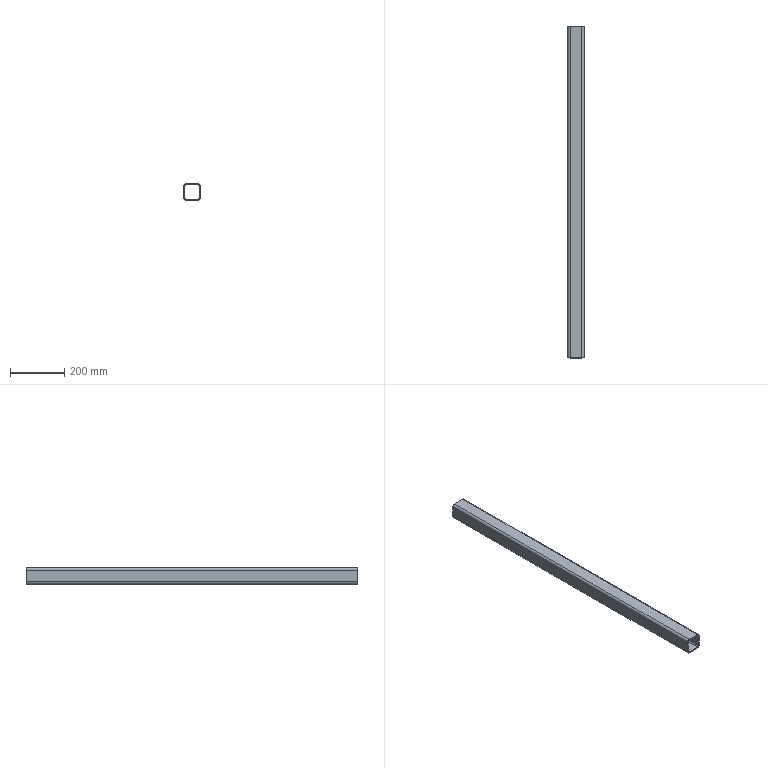Part | SolidWorks | features BaseBody 1 | 1 solid | 18 faces | box 60 x 1220 x 60 mm | volume 1042852 mm3 | plane 10 | cylinder 8 | commonest cylinder face diameters 8 x4 16 x4
STEP:
#1=CARTESIAN_POINT('',(-644.,2432.,552.));
#2=VERTEX_POINT('',#1);
#3=CARTESIAN_POINT('',(-644.,2432.,508.));
#4=VERTEX_POINT('',#3);
#5=CARTESIAN_POINT('',(-644.,2432.,508.));
#6=DIRECTION('',(0.,0.,-1.));
#7=VECTOR('',#6,1000.);
#8=LINE('',#5,#7);
#9=EDGE_CURVE('',#2,#4,#8,.T.);
#10=ORIENTED_EDGE('',*,*,#9,.T.);
#11=CARTESIAN_POINT('',(-644.,1212.,508.));
#12=VERTEX_POINT('',#11);
#13=CARTESIAN_POINT('',(-644.,2462.,508.));
#14=DIRECTION('',(0.,-1.,0.));
#15=VECTOR('',#14,1000.);
#16=LINE('',#13,#15);
#17=EDGE_CURVE('',#4,#12,#16,.T.);
#18=ORIENTED_EDGE('',*,*,#17,.T.);
#19=CARTESIAN_POINT('',(-644.,1212.,552.));
#20=VERTEX_POINT('',#19);
#21=CARTESIAN_POINT('',(-644.,1212.,508.));
#22=DIRECTION('',(0.,0.,1.));
#23=VECTOR('',#22,1000.);
#24=LINE('',#21,#23);
#25=EDGE_CURVE('',#12,#20,#24,.T.);
#26=ORIENTED_EDGE('',*,*,#25,.T.);
#27=CARTESIAN_POINT('',(-644.,2462.,552.));
#28=DIRECTION('',(0.,1.,0.));
#29=VECTOR('',#28,1000.);
#30=LINE('',#27,#29);
#31=EDGE_CURVE('',#20,#2,#30,.T.);
#32=ORIENTED_EDGE('',*,*,#31,.T.);
#33=EDGE_LOOP('',(#10,#18,#26,#32));
#34=FACE_OUTER_BOUND('',#33,.T.);
#35=CARTESIAN_POINT('',(-644.,2462.,508.));
#36=DIRECTION('',(-1.,0.,0.));
#37=DIRECTION('',(0.,0.,1.));
#38=AXIS2_PLACEMENT_3D('',#35,#36,#37);
#39=PLANE('',#38);
#40=ADVANCED_FACE('',(#34),#39,.T.);
#41=ORIENTED_EDGE('',*,*,#17,.F.);
#42=CARTESIAN_POINT('',(-648.,2432.,504.));
#43=VERTEX_POINT('',#42);
#44=CARTESIAN_POINT('',(-648.,2432.,508.));
#45=DIRECTION('',(0.,-1.,0.));
#46=DIRECTION('',(0.,0.,-1.));
#47=AXIS2_PLACEMENT_3D('',#44,#45,#46);
#48=CIRCLE('',#47,4.);
#49=EDGE_CURVE('',#43,#4,#48,.T.);
#50=ORIENTED_EDGE('',*,*,#49,.F.);
#51=CARTESIAN_POINT('',(-648.,1212.,504.));
#52=VERTEX_POINT('',#51);
#53=CARTESIAN_POINT('',(-648.,2462.,504.));
#54=DIRECTION('',(0.,1.,0.));
#55=VECTOR('',#54,1000.);
#56=LINE('',#53,#55);
#57=EDGE_CURVE('',#52,#43,#56,.T.);
#58=ORIENTED_EDGE('',*,*,#57,.F.);
#59=CARTESIAN_POINT('',(-648.,1212.,508.));
#60=DIRECTION('',(0.,1.,0.));
#61=DIRECTION('',(0.,0.,-1.));
#62=AXIS2_PLACEMENT_3D('',#59,#60,#61);
#63=CIRCLE('',#62,4.);
#64=EDGE_CURVE('',#12,#52,#63,.T.);
#65=ORIENTED_EDGE('',*,*,#64,.F.);
#66=EDGE_LOOP('',(#41,#50,#58,#65));
#67=FACE_OUTER_BOUND('',#66,.T.);
#68=CARTESIAN_POINT('',(-648.,2462.,508.));
#69=DIRECTION('',(0.,-1.,0.));
#70=DIRECTION('',(0.,0.,-1.));
#71=AXIS2_PLACEMENT_3D('',#68,#69,#70);
#72=CYLINDRICAL_SURFACE('',#71,4.);
#73=ADVANCED_FACE('',(#67),#72,.F.);
#74=CARTESIAN_POINT('',(-648.,2432.,556.));
#75=VERTEX_POINT('',#74);
#76=CARTESIAN_POINT('',(-648.,2432.,552.));
#77=DIRECTION('',(0.,-1.,0.));
#78=DIRECTION('',(0.,0.,-1.));
#79=AXIS2_PLACEMENT_3D('',#76,#77,#78);
#80=CIRCLE('',#79,4.);
#81=EDGE_CURVE('',#2,#75,#80,.T.);
#82=ORIENTED_EDGE('',*,*,#81,.T.);
#83=CARTESIAN_POINT('',(-692.,2432.,556.));
#84=VERTEX_POINT('',#83);
#85=CARTESIAN_POINT('',(-648.,2432.,556.));
#86=DIRECTION('',(-1.,0.,0.));
#87=VECTOR('',#86,1000.);
#88=LINE('',#85,#87);
#89=EDGE_CURVE('',#75,#84,#88,.T.);
#90=ORIENTED_EDGE('',*,*,#89,.T.);
#91=CARTESIAN_POINT('',(-696.,2432.,552.));
#92=VERTEX_POINT('',#91);
#93=CARTESIAN_POINT('',(-692.,2432.,552.));
#94=DIRECTION('',(0.,-1.,0.));
#95=DIRECTION('',(0.,0.,-1.));
#96=AXIS2_PLACEMENT_3D('',#93,#94,#95);
#97=CIRCLE('',#96,4.);
#98=EDGE_CURVE('',#84,#92,#97,.T.);
#99=ORIENTED_EDGE('',*,*,#98,.T.);
#100=CARTESIAN_POINT('',(-696.,2432.,508.));
#101=VERTEX_POINT('',#100);
#102=CARTESIAN_POINT('',(-696.,2432.,-1270.));
#103=DIRECTION('',(0.,0.,-1.));
#104=VECTOR('',#103,1000.);
#105=LINE('',#102,#104);
#106=EDGE_CURVE('',#92,#101,#105,.T.);
#107=ORIENTED_EDGE('',*,*,#106,.T.);
#108=CARTESIAN_POINT('',(-692.,2432.,504.));
#109=VERTEX_POINT('',#108);
#110=CARTESIAN_POINT('',(-692.,2432.,508.));
#111=DIRECTION('',(0.,-1.,0.));
#112=DIRECTION('',(0.,0.,-1.));
#113=AXIS2_PLACEMENT_3D('',#110,#111,#112);
#114=CIRCLE('',#113,4.);
#115=EDGE_CURVE('',#101,#109,#114,.T.);
#116=ORIENTED_EDGE('',*,*,#115,.T.);
#117=CARTESIAN_POINT('',(-648.,2432.,504.));
#118=DIRECTION('',(1.,0.,0.));
#119=VECTOR('',#118,1000.);
#120=LINE('',#117,#119);
#121=EDGE_CURVE('',#109,#43,#120,.T.);
#122=ORIENTED_EDGE('',*,*,#121,.T.);
#123=ORIENTED_EDGE('',*,*,#49,.T.);
#124=ORIENTED_EDGE('',*,*,#9,.F.);
#125=EDGE_LOOP('',(#82,#90,#99,#107,#116,#122,#123,#124));
#126=FACE_BOUND('',#125,.T.);
#127=CARTESIAN_POINT('',(-700.,2432.,508.));
#128=VERTEX_POINT('',#127);
#129=CARTESIAN_POINT('',(-700.,2432.,552.));
#130=VERTEX_POINT('',#129);
#131=CARTESIAN_POINT('',(-700.,2432.,-1270.));
#132=DIRECTION('',(0.,0.,1.));
#133=VECTOR('',#132,1000.);
#134=LINE('',#131,#133);
#135=EDGE_CURVE('',#128,#130,#134,.T.);
#136=ORIENTED_EDGE('',*,*,#135,.T.);
#137=CARTESIAN_POINT('',(-692.,2432.,560.));
#138=VERTEX_POINT('',#137);
#139=CARTESIAN_POINT('',(-692.,2432.,552.));
#140=DIRECTION('',(0.,1.,0.));
#141=DIRECTION('',(0.,0.,-1.));
#142=AXIS2_PLACEMENT_3D('',#139,#140,#141);
#143=CIRCLE('',#142,8.);
#144=EDGE_CURVE('',#130,#138,#143,.T.);
#145=ORIENTED_EDGE('',*,*,#144,.T.);
#146=CARTESIAN_POINT('',(-648.,2432.,560.));
#147=VERTEX_POINT('',#146);
#148=CARTESIAN_POINT('',(-648.,2432.,560.));
#149=DIRECTION('',(1.,0.,0.));
#150=VECTOR('',#149,1000.);
#151=LINE('',#148,#150);
#152=EDGE_CURVE('',#138,#147,#151,.T.);
#153=ORIENTED_EDGE('',*,*,#152,.T.);
#154=CARTESIAN_POINT('',(-640.,2432.,552.));
#155=VERTEX_POINT('',#154);
#156=CARTESIAN_POINT('',(-648.,2432.,552.));
#157=DIRECTION('',(0.,1.,0.));
#158=DIRECTION('',(0.,0.,-1.));
#159=AXIS2_PLACEMENT_3D('',#156,#157,#158);
#160=CIRCLE('',#159,8.);
#161=EDGE_CURVE('',#147,#155,#160,.T.);
#162=ORIENTED_EDGE('',*,*,#161,.T.);
#163=CARTESIAN_POINT('',(-640.,2432.,508.));
#164=VERTEX_POINT('',#163);
#165=CARTESIAN_POINT('',(-640.,2432.,-1270.));
#166=DIRECTION('',(0.,0.,-1.));
#167=VECTOR('',#166,1000.);
#168=LINE('',#165,#167);
#169=EDGE_CURVE('',#155,#164,#168,.T.);
#170=ORIENTED_EDGE('',*,*,#169,.T.);
#171=CARTESIAN_POINT('',(-648.,2432.,500.));
#172=VERTEX_POINT('',#171);
#173=CARTESIAN_POINT('',(-648.,2432.,508.));
#174=DIRECTION('',(0.,1.,0.));
#175=DIRECTION('',(0.,0.,-1.));
#176=AXIS2_PLACEMENT_3D('',#173,#174,#175);
#177=CIRCLE('',#176,8.);
#178=EDGE_CURVE('',#164,#172,#177,.T.);
#179=ORIENTED_EDGE('',*,*,#178,.T.);
#180=CARTESIAN_POINT('',(-692.,2432.,500.));
#181=VERTEX_POINT('',#180);
#182=CARTESIAN_POINT('',(-648.,2432.,500.));
#183=DIRECTION('',(-1.,0.,0.));
#184=VECTOR('',#183,1000.);
#185=LINE('',#182,#184);
#186=EDGE_CURVE('',#172,#181,#185,.T.);
#187=ORIENTED_EDGE('',*,*,#186,.T.);
#188=CARTESIAN_POINT('',(-692.,2432.,508.));
#189=DIRECTION('',(0.,1.,0.));
#190=DIRECTION('',(0.,0.,-1.));
#191=AXIS2_PLACEMENT_3D('',#188,#189,#190);
#192=CIRCLE('',#191,8.);
#193=EDGE_CURVE('',#181,#128,#192,.T.);
#194=ORIENTED_EDGE('',*,*,#193,.T.);
#195=EDGE_LOOP('',(#136,#145,#153,#162,#170,#179,#187,#194));
#196=FACE_OUTER_BOUND('',#195,.T.);
#197=CARTESIAN_POINT('',(-648.,2432.,-1270.));
#198=DIRECTION('',(0.,1.,0.));
#199=DIRECTION('',(0.,0.,1.));
#200=AXIS2_PLACEMENT_3D('',#197,#198,#199);
#201=PLANE('',#200);
#202=ADVANCED_FACE('',(#126,#196),#201,.T.);
#203=CARTESIAN_POINT('',(-648.,1212.,556.));
#204=VERTEX_POINT('',#203);
#205=CARTESIAN_POINT('',(-648.,2462.,556.));
#206=DIRECTION('',(0.,-1.,0.));
#207=VECTOR('',#206,1000.);
#208=LINE('',#205,#207);
#209=EDGE_CURVE('',#75,#204,#208,.T.);
#210=ORIENTED_EDGE('',*,*,#209,.F.);
#211=ORIENTED_EDGE('',*,*,#81,.F.);
#212=ORIENTED_EDGE('',*,*,#31,.F.);
#213=CARTESIAN_POINT('',(-648.,1212.,552.));
#214=DIRECTION('',(0.,1.,0.));
#215=DIRECTION('',(0.,0.,-1.));
#216=AXIS2_PLACEMENT_3D('',#213,#214,#215);
#217=CIRCLE('',#216,4.);
#218=EDGE_CURVE('',#204,#20,#217,.T.);
#219=ORIENTED_EDGE('',*,*,#218,.F.);
#220=EDGE_LOOP('',(#210,#211,#212,#219));
#221=FACE_OUTER_BOUND('',#220,.T.);
#222=CARTESIAN_POINT('',(-648.,2462.,552.));
#223=DIRECTION('',(0.,-1.,0.));
#224=DIRECTION('',(0.,0.,-1.));
#225=AXIS2_PLACEMENT_3D('',#222,#223,#224);
#226=CYLINDRICAL_SURFACE('',#225,4.);
#227=ADVANCED_FACE('',(#221),#226,.F.);
#228=CARTESIAN_POINT('',(-692.,1212.,556.));
#229=VERTEX_POINT('',#228);
#230=CARTESIAN_POINT('',(-640.,1212.,556.));
#231=DIRECTION('',(1.,0.,0.));
#232=VECTOR('',#231,1000.);
#233=LINE('',#230,#232);
#234=EDGE_CURVE('',#229,#204,#233,.T.);
#235=ORIENTED_EDGE('',*,*,#234,.T.);
#236=ORIENTED_EDGE('',*,*,#218,.T.);
#237=ORIENTED_EDGE('',*,*,#25,.F.);
#238=ORIENTED_EDGE('',*,*,#64,.T.);
#239=CARTESIAN_POINT('',(-692.,1212.,504.));
#240=VERTEX_POINT('',#239);
#241=CARTESIAN_POINT('',(-640.,1212.,504.));
#242=DIRECTION('',(-1.,0.,0.));
#243=VECTOR('',#242,1000.);
#244=LINE('',#241,#243);
#245=EDGE_CURVE('',#52,#240,#244,.T.);
#246=ORIENTED_EDGE('',*,*,#245,.T.);
#247=CARTESIAN_POINT('',(-696.,1212.,508.));
#248=VERTEX_POINT('',#247);
#249=CARTESIAN_POINT('',(-692.,1212.,508.));
#250=DIRECTION('',(0.,1.,0.));
#251=DIRECTION('',(0.,0.,-1.));
#252=AXIS2_PLACEMENT_3D('',#249,#250,#251);
#253=CIRCLE('',#252,4.);
#254=EDGE_CURVE('',#240,#248,#253,.T.);
#255=ORIENTED_EDGE('',*,*,#254,.T.);
#256=CARTESIAN_POINT('',(-696.,1212.,552.));
#257=VERTEX_POINT('',#256);
#258=CARTESIAN_POINT('',(-696.,1212.,530.));
#259=DIRECTION('',(0.,0.,1.));
#260=VECTOR('',#259,1000.);
#261=LINE('',#258,#260);
#262=EDGE_CURVE('',#248,#257,#261,.T.);
#263=ORIENTED_EDGE('',*,*,#262,.T.);
#264=CARTESIAN_POINT('',(-692.,1212.,552.));
#265=DIRECTION('',(0.,1.,0.));
#266=DIRECTION('',(0.,0.,-1.));
#267=AXIS2_PLACEMENT_3D('',#264,#265,#266);
#268=CIRCLE('',#267,4.);
#269=EDGE_CURVE('',#257,#229,#268,.T.);
#270=ORIENTED_EDGE('',*,*,#269,.T.);
#271=EDGE_LOOP('',(#235,#236,#237,#238,#246,#255,#263,#270));
#272=FACE_BOUND('',#271,.T.);
#273=CARTESIAN_POINT('',(-640.,1212.,552.));
#274=VERTEX_POINT('',#273);
#275=CARTESIAN_POINT('',(-648.,1212.,560.));
#276=VERTEX_POINT('',#275);
#277=CARTESIAN_POINT('',(-648.,1212.,552.));
#278=DIRECTION('',(0.,-1.,0.));
#279=DIRECTION('',(0.,0.,-1.));
#280=AXIS2_PLACEMENT_3D('',#277,#278,#279);
#281=CIRCLE('',#280,8.);
#282=EDGE_CURVE('',#274,#276,#281,.T.);
#283=ORIENTED_EDGE('',*,*,#282,.T.);
#284=CARTESIAN_POINT('',(-692.,1212.,560.));
#285=VERTEX_POINT('',#284);
#286=CARTESIAN_POINT('',(-640.,1212.,560.));
#287=DIRECTION('',(-1.,0.,0.));
#288=VECTOR('',#287,1000.);
#289=LINE('',#286,#288);
#290=EDGE_CURVE('',#276,#285,#289,.T.);
#291=ORIENTED_EDGE('',*,*,#290,.T.);
#292=CARTESIAN_POINT('',(-700.,1212.,552.));
#293=VERTEX_POINT('',#292);
#294=CARTESIAN_POINT('',(-692.,1212.,552.));
#295=DIRECTION('',(0.,-1.,0.));
#296=DIRECTION('',(0.,0.,-1.));
#297=AXIS2_PLACEMENT_3D('',#294,#295,#296);
#298=CIRCLE('',#297,8.);
#299=EDGE_CURVE('',#285,#293,#298,.T.);
#300=ORIENTED_EDGE('',*,*,#299,.T.);
#301=CARTESIAN_POINT('',(-700.,1212.,508.));
#302=VERTEX_POINT('',#301);
#303=CARTESIAN_POINT('',(-700.,1212.,530.));
#304=DIRECTION('',(0.,0.,-1.));
#305=VECTOR('',#304,1000.);
#306=LINE('',#303,#305);
#307=EDGE_CURVE('',#293,#302,#306,.T.);
#308=ORIENTED_EDGE('',*,*,#307,.T.);
#309=CARTESIAN_POINT('',(-692.,1212.,500.));
#310=VERTEX_POINT('',#309);
#311=CARTESIAN_POINT('',(-692.,1212.,508.));
#312=DIRECTION('',(0.,-1.,0.));
#313=DIRECTION('',(0.,0.,-1.));
#314=AXIS2_PLACEMENT_3D('',#311,#312,#313);
#315=CIRCLE('',#314,8.);
#316=EDGE_CURVE('',#302,#310,#315,.T.);
#317=ORIENTED_EDGE('',*,*,#316,.T.);
#318=CARTESIAN_POINT('',(-648.,1212.,500.));
#319=VERTEX_POINT('',#318);
#320=CARTESIAN_POINT('',(-640.,1212.,500.));
#321=DIRECTION('',(1.,0.,0.));
#322=VECTOR('',#321,1000.);
#323=LINE('',#320,#322);
#324=EDGE_CURVE('',#310,#319,#323,.T.);
#325=ORIENTED_EDGE('',*,*,#324,.T.);
#326=CARTESIAN_POINT('',(-640.,1212.,508.));
#327=VERTEX_POINT('',#326);
#328=CARTESIAN_POINT('',(-648.,1212.,508.));
#329=DIRECTION('',(0.,-1.,0.));
#330=DIRECTION('',(0.,0.,-1.));
#331=AXIS2_PLACEMENT_3D('',#328,#329,#330);
#332=CIRCLE('',#331,8.);
#333=EDGE_CURVE('',#319,#327,#332,.T.);
#334=ORIENTED_EDGE('',*,*,#333,.T.);
#335=CARTESIAN_POINT('',(-640.,1212.,530.));
#336=DIRECTION('',(0.,0.,1.));
#337=VECTOR('',#336,1000.);
#338=LINE('',#335,#337);
#339=EDGE_CURVE('',#327,#274,#338,.T.);
#340=ORIENTED_EDGE('',*,*,#339,.T.);
#341=EDGE_LOOP('',(#283,#291,#300,#308,#317,#325,#334,#340));
#342=FACE_OUTER_BOUND('',#341,.T.);
#343=CARTESIAN_POINT('',(-640.,1212.,530.));
#344=DIRECTION('',(0.,-1.,0.));
#345=DIRECTION('',(0.,0.,-1.));
#346=AXIS2_PLACEMENT_3D('',#343,#344,#345);
#347=PLANE('',#346);
#348=ADVANCED_FACE('',(#272,#342),#347,.T.);
#349=ORIENTED_EDGE('',*,*,#121,.F.);
#350=CARTESIAN_POINT('',(-692.,2462.,504.));
#351=DIRECTION('',(0.,-1.,0.));
#352=VECTOR('',#351,1000.);
#353=LINE('',#350,#352);
#354=EDGE_CURVE('',#109,#240,#353,.T.);
#355=ORIENTED_EDGE('',*,*,#354,.T.);
#356=ORIENTED_EDGE('',*,*,#245,.F.);
#357=ORIENTED_EDGE('',*,*,#57,.T.);
#358=EDGE_LOOP('',(#349,#355,#356,#357));
#359=FACE_OUTER_BOUND('',#358,.T.);
#360=CARTESIAN_POINT('',(-648.,2462.,504.));
#361=DIRECTION('',(0.,0.,1.));
#362=DIRECTION('',(1.,0.,0.));
#363=AXIS2_PLACEMENT_3D('',#360,#361,#362);
#364=PLANE('',#363);
#365=ADVANCED_FACE('',(#359),#364,.T.);
#366=ORIENTED_EDGE('',*,*,#89,.F.);
#367=ORIENTED_EDGE('',*,*,#209,.T.);
#368=ORIENTED_EDGE('',*,*,#234,.F.);
#369=CARTESIAN_POINT('',(-692.,2462.,556.));
#370=DIRECTION('',(0.,1.,0.));
#371=VECTOR('',#370,1000.);
#372=LINE('',#369,#371);
#373=EDGE_CURVE('',#229,#84,#372,.T.);
#374=ORIENTED_EDGE('',*,*,#373,.T.);
#375=EDGE_LOOP('',(#366,#367,#368,#374));
#376=FACE_OUTER_BOUND('',#375,.T.);
#377=CARTESIAN_POINT('',(-692.,2462.,556.));
#378=DIRECTION('',(0.,0.,-1.));
#379=DIRECTION('',(-1.,0.,0.));
#380=AXIS2_PLACEMENT_3D('',#377,#378,#379);
#381=PLANE('',#380);
#382=ADVANCED_FACE('',(#376),#381,.T.);
#383=ORIENTED_EDGE('',*,*,#354,.F.);
#384=ORIENTED_EDGE('',*,*,#115,.F.);
#385=CARTESIAN_POINT('',(-696.,2462.,508.));
#386=DIRECTION('',(0.,1.,0.));
#387=VECTOR('',#386,1000.);
#388=LINE('',#385,#387);
#389=EDGE_CURVE('',#248,#101,#388,.T.);
#390=ORIENTED_EDGE('',*,*,#389,.F.);
#391=ORIENTED_EDGE('',*,*,#254,.F.);
#392=EDGE_LOOP('',(#383,#384,#390,#391));
#393=FACE_OUTER_BOUND('',#392,.T.);
#394=CARTESIAN_POINT('',(-692.,2462.,508.));
#395=DIRECTION('',(0.,-1.,0.));
#396=DIRECTION('',(0.,0.,-1.));
#397=AXIS2_PLACEMENT_3D('',#394,#395,#396);
#398=CYLINDRICAL_SURFACE('',#397,4.);
#399=ADVANCED_FACE('',(#393),#398,.F.);
#400=ORIENTED_EDGE('',*,*,#106,.F.);
#401=CARTESIAN_POINT('',(-696.,2462.,552.));
#402=DIRECTION('',(0.,-1.,0.));
#403=VECTOR('',#402,1000.);
#404=LINE('',#401,#403);
#405=EDGE_CURVE('',#92,#257,#404,.T.);
#406=ORIENTED_EDGE('',*,*,#405,.T.);
#407=ORIENTED_EDGE('',*,*,#262,.F.);
#408=ORIENTED_EDGE('',*,*,#389,.T.);
#409=EDGE_LOOP('',(#400,#406,#407,#408));
#410=FACE_OUTER_BOUND('',#409,.T.);
#411=CARTESIAN_POINT('',(-696.,2462.,552.));
#412=DIRECTION('',(1.,0.,0.));
#413=DIRECTION('',(0.,0.,-1.));
#414=AXIS2_PLACEMENT_3D('',#411,#412,#413);
#415=PLANE('',#414);
#416=ADVANCED_FACE('',(#410),#415,.T.);
#417=ORIENTED_EDGE('',*,*,#405,.F.);
#418=ORIENTED_EDGE('',*,*,#98,.F.);
#419=ORIENTED_EDGE('',*,*,#373,.F.);
#420=ORIENTED_EDGE('',*,*,#269,.F.);
#421=EDGE_LOOP('',(#417,#418,#419,#420));
#422=FACE_OUTER_BOUND('',#421,.T.);
#423=CARTESIAN_POINT('',(-692.,2462.,552.));
#424=DIRECTION('',(0.,-1.,0.));
#425=DIRECTION('',(0.,0.,-1.));
#426=AXIS2_PLACEMENT_3D('',#423,#424,#425);
#427=CYLINDRICAL_SURFACE('',#426,4.);
#428=ADVANCED_FACE('',(#422),#427,.F.);
#429=CARTESIAN_POINT('',(-700.,2462.,552.));
#430=DIRECTION('',(0.,-1.,0.));
#431=VECTOR('',#430,1000.);
#432=LINE('',#429,#431);
#433=EDGE_CURVE('',#130,#293,#432,.T.);
#434=ORIENTED_EDGE('',*,*,#433,.T.);
#435=ORIENTED_EDGE('',*,*,#299,.F.);
#436=CARTESIAN_POINT('',(-692.,2462.,560.));
#437=DIRECTION('',(0.,1.,0.));
#438=VECTOR('',#437,1000.);
#439=LINE('',#436,#438);
#440=EDGE_CURVE('',#285,#138,#439,.T.);
#441=ORIENTED_EDGE('',*,*,#440,.T.);
#442=ORIENTED_EDGE('',*,*,#144,.F.);
#443=EDGE_LOOP('',(#434,#435,#441,#442));
#444=FACE_OUTER_BOUND('',#443,.T.);
#445=CARTESIAN_POINT('',(-692.,2462.,552.));
#446=DIRECTION('',(0.,-1.,0.));
#447=DIRECTION('',(0.,0.,-1.));
#448=AXIS2_PLACEMENT_3D('',#445,#446,#447);
#449=CYLINDRICAL_SURFACE('',#448,8.);
#450=ADVANCED_FACE('',(#444),#449,.T.);
#451=ORIENTED_EDGE('',*,*,#135,.F.);
#452=CARTESIAN_POINT('',(-700.,2462.,508.));
#453=DIRECTION('',(0.,1.,0.));
#454=VECTOR('',#453,1000.);
#455=LINE('',#452,#454);
#456=EDGE_CURVE('',#302,#128,#455,.T.);
#457=ORIENTED_EDGE('',*,*,#456,.F.);
#458=ORIENTED_EDGE('',*,*,#307,.F.);
#459=ORIENTED_EDGE('',*,*,#433,.F.);
#460=EDGE_LOOP('',(#451,#457,#458,#459));
#461=FACE_OUTER_BOUND('',#460,.T.);
#462=CARTESIAN_POINT('',(-700.,2462.,552.));
#463=DIRECTION('',(1.,0.,0.));
#464=DIRECTION('',(0.,0.,-1.));
#465=AXIS2_PLACEMENT_3D('',#462,#463,#464);
#466=PLANE('',#465);
#467=ADVANCED_FACE('',(#461),#466,.F.);
#468=CARTESIAN_POINT('',(-692.,2462.,500.));
#469=DIRECTION('',(0.,-1.,0.));
#470=VECTOR('',#469,1000.);
#471=LINE('',#468,#470);
#472=EDGE_CURVE('',#181,#310,#471,.T.);
#473=ORIENTED_EDGE('',*,*,#472,.T.);
#474=ORIENTED_EDGE('',*,*,#316,.F.);
#475=ORIENTED_EDGE('',*,*,#456,.T.);
#476=ORIENTED_EDGE('',*,*,#193,.F.);
#477=EDGE_LOOP('',(#473,#474,#475,#476));
#478=FACE_OUTER_BOUND('',#477,.T.);
#479=CARTESIAN_POINT('',(-692.,2462.,508.));
#480=DIRECTION('',(0.,-1.,0.));
#481=DIRECTION('',(0.,0.,-1.));
#482=AXIS2_PLACEMENT_3D('',#479,#480,#481);
#483=CYLINDRICAL_SURFACE('',#482,8.);
#484=ADVANCED_FACE('',(#478),#483,.T.);
#485=ORIENTED_EDGE('',*,*,#186,.F.);
#486=CARTESIAN_POINT('',(-648.,2462.,500.));
#487=DIRECTION('',(0.,1.,0.));
#488=VECTOR('',#487,1000.);
#489=LINE('',#486,#488);
#490=EDGE_CURVE('',#319,#172,#489,.T.);
#491=ORIENTED_EDGE('',*,*,#490,.F.);
#492=ORIENTED_EDGE('',*,*,#324,.F.);
#493=ORIENTED_EDGE('',*,*,#472,.F.);
#494=EDGE_LOOP('',(#485,#491,#492,#493));
#495=FACE_OUTER_BOUND('',#494,.T.);
#496=CARTESIAN_POINT('',(-648.,2462.,500.));
#497=DIRECTION('',(0.,0.,1.));
#498=DIRECTION('',(1.,0.,0.));
#499=AXIS2_PLACEMENT_3D('',#496,#497,#498);
#500=PLANE('',#499);
#501=ADVANCED_FACE('',(#495),#500,.F.);
#502=CARTESIAN_POINT('',(-640.,2462.,508.));
#503=DIRECTION('',(0.,-1.,0.));
#504=VECTOR('',#503,1000.);
#505=LINE('',#502,#504);
#506=EDGE_CURVE('',#164,#327,#505,.T.);
#507=ORIENTED_EDGE('',*,*,#506,.T.);
#508=ORIENTED_EDGE('',*,*,#333,.F.);
#509=ORIENTED_EDGE('',*,*,#490,.T.);
#510=ORIENTED_EDGE('',*,*,#178,.F.);
#511=EDGE_LOOP('',(#507,#508,#509,#510));
#512=FACE_OUTER_BOUND('',#511,.T.);
#513=CARTESIAN_POINT('',(-648.,2462.,508.));
#514=DIRECTION('',(0.,-1.,0.));
#515=DIRECTION('',(0.,0.,-1.));
#516=AXIS2_PLACEMENT_3D('',#513,#514,#515);
#517=CYLINDRICAL_SURFACE('',#516,8.);
#518=ADVANCED_FACE('',(#512),#517,.T.);
#519=ORIENTED_EDGE('',*,*,#169,.F.);
#520=CARTESIAN_POINT('',(-640.,2462.,552.));
#521=DIRECTION('',(0.,1.,0.));
#522=VECTOR('',#521,1000.);
#523=LINE('',#520,#522);
#524=EDGE_CURVE('',#274,#155,#523,.T.);
#525=ORIENTED_EDGE('',*,*,#524,.F.);
#526=ORIENTED_EDGE('',*,*,#339,.F.);
#527=ORIENTED_EDGE('',*,*,#506,.F.);
#528=EDGE_LOOP('',(#519,#525,#526,#527));
#529=FACE_OUTER_BOUND('',#528,.T.);
#530=CARTESIAN_POINT('',(-640.,2462.,508.));
#531=DIRECTION('',(-1.,0.,0.));
#532=DIRECTION('',(0.,0.,1.));
#533=AXIS2_PLACEMENT_3D('',#530,#531,#532);
#534=PLANE('',#533);
#535=ADVANCED_FACE('',(#529),#534,.F.);
#536=CARTESIAN_POINT('',(-648.,2462.,560.));
#537=DIRECTION('',(0.,-1.,0.));
#538=VECTOR('',#537,1000.);
#539=LINE('',#536,#538);
#540=EDGE_CURVE('',#147,#276,#539,.T.);
#541=ORIENTED_EDGE('',*,*,#540,.T.);
#542=ORIENTED_EDGE('',*,*,#282,.F.);
#543=ORIENTED_EDGE('',*,*,#524,.T.);
#544=ORIENTED_EDGE('',*,*,#161,.F.);
#545=EDGE_LOOP('',(#541,#542,#543,#544));
#546=FACE_OUTER_BOUND('',#545,.T.);
#547=CARTESIAN_POINT('',(-648.,2462.,552.));
#548=DIRECTION('',(0.,-1.,0.));
#549=DIRECTION('',(0.,0.,-1.));
#550=AXIS2_PLACEMENT_3D('',#547,#548,#549);
#551=CYLINDRICAL_SURFACE('',#550,8.);
#552=ADVANCED_FACE('',(#546),#551,.T.);
#553=ORIENTED_EDGE('',*,*,#152,.F.);
#554=ORIENTED_EDGE('',*,*,#440,.F.);
#555=ORIENTED_EDGE('',*,*,#290,.F.);
#556=ORIENTED_EDGE('',*,*,#540,.F.);
#557=EDGE_LOOP('',(#553,#554,#555,#556));
#558=FACE_OUTER_BOUND('',#557,.T.);
#559=CARTESIAN_POINT('',(-692.,2462.,560.));
#560=DIRECTION('',(0.,0.,-1.));
#561=DIRECTION('',(-1.,0.,0.));
#562=AXIS2_PLACEMENT_3D('',#559,#560,#561);
#563=PLANE('',#562);
#564=ADVANCED_FACE('',(#558),#563,.F.);
#565=CLOSED_SHELL('',(#40,#73,#202,#227,#348,#365,#382,#399,#416,#428,#450,#467,#484,#501,#518,#535,#552,#564));
#566=MANIFOLD_SOLID_BREP('',#565);
#567=CARTESIAN_POINT('',(0.,0.,0.));
#568=DIRECTION('',(0.,0.,1.));
#569=DIRECTION('',(1.,0.,0.));
#570=AXIS2_PLACEMENT_3D('',#567,#568,#569);
#571=(LENGTH_UNIT()NAMED_UNIT(*)SI_UNIT(.MILLI.,.METRE.));
#572=UNCERTAINTY_MEASURE_WITH_UNIT(LENGTH_MEASURE(0.00001),#571,'','');
#573=(NAMED_UNIT(*)PLANE_ANGLE_UNIT()SI_UNIT($,.RADIAN.));
#574=(NAMED_UNIT(*)SI_UNIT($,.STERADIAN.)SOLID_ANGLE_UNIT());
#575=(GEOMETRIC_REPRESENTATION_CONTEXT(3)GLOBAL_UNCERTAINTY_ASSIGNED_CONTEXT((#572))GLOBAL_UNIT_ASSIGNED_CONTEXT((#571,#573,#574))REPRESENTATION_CONTEXT('',''));
#576=ADVANCED_BREP_SHAPE_REPRESENTATION('',(#566,#570),#575);